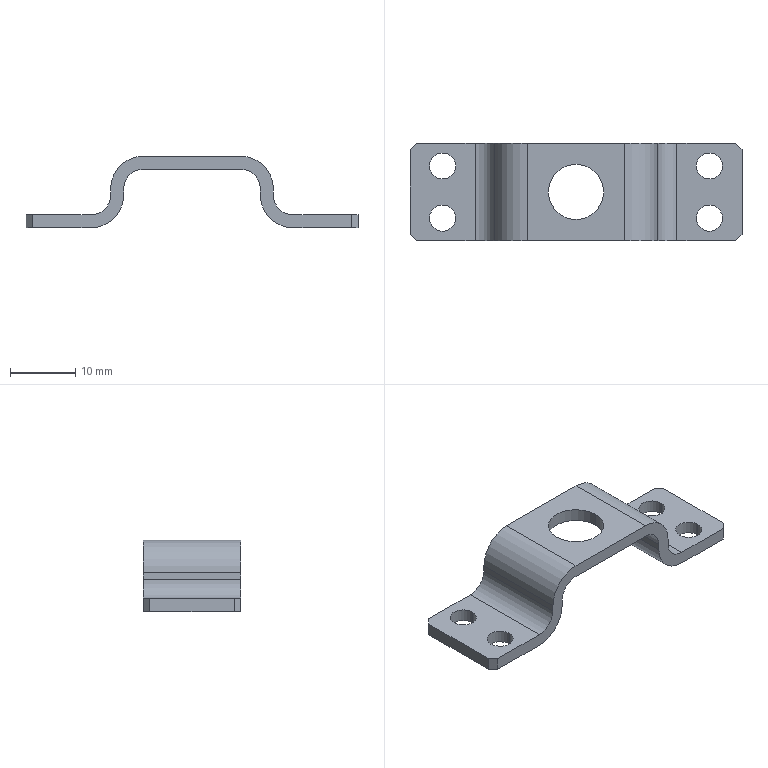Part | STEP file | Jig prox plate | 1 solid | 36 faces | box 51 x 15 x 11 mm | volume 1646 mm3 | cylinder 18 | plane 18 | commonest cylinder face diameters 4 x8 6 x4 10 x4 8.5 x2